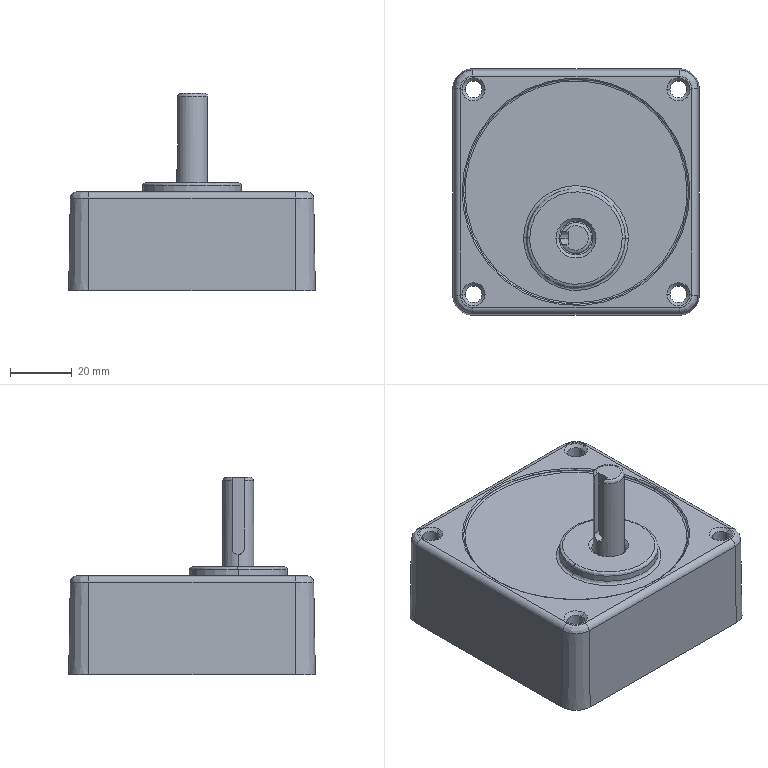Part | SolidWorks | features BaseBody 1 | 1 solid | 67 faces | box 80 x 80 x 64 mm | volume 187976 mm3 | cylinder 22 | cone 18 | plane 14 | spline 13 | commonest cylinder face diameters 5.5 x8 4 x6 10 x2 11 x2 32 x2 73 x2